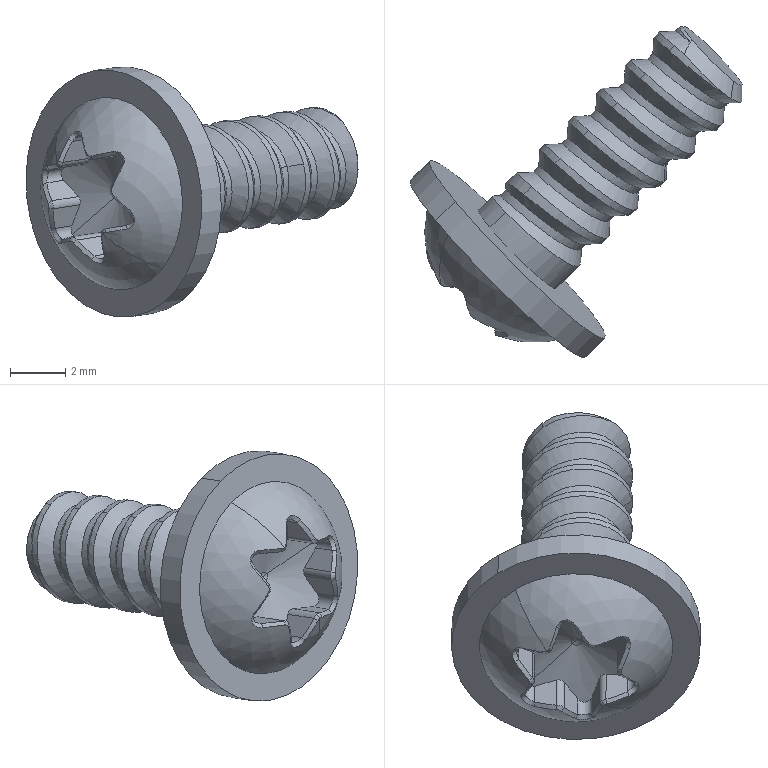Part | SolidWorks | features BaseBody 1 | 1 solid | 86 faces | box 12.021 x 11.98 x 9.055 mm | volume 194.201 mm3 | cylinder 27 | spline 23 | cone 17 | plane 15 | sphere 4 | commonest cylinder face diameters 4 x13 0.6 x12 9 x2